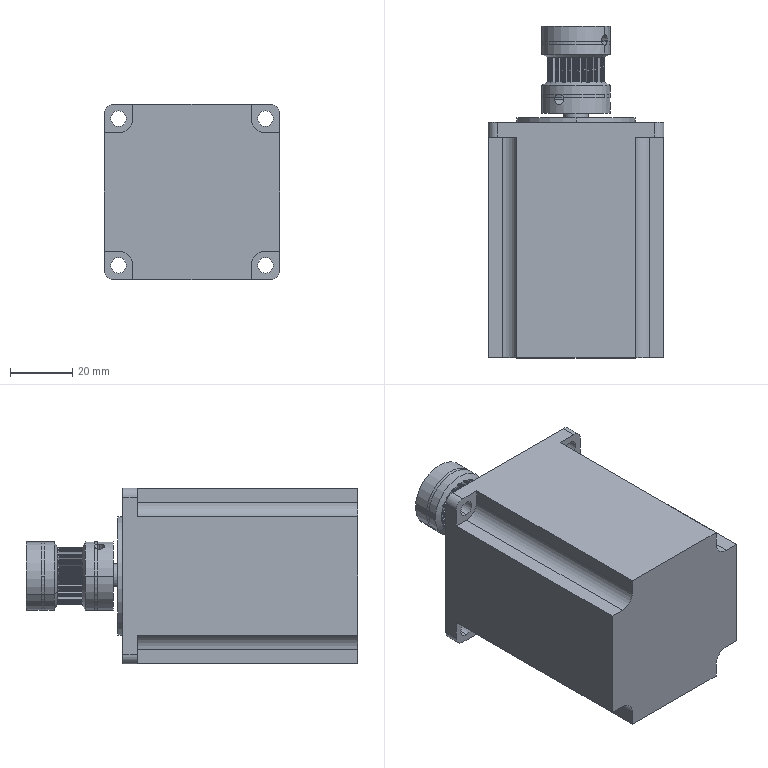Part | SolidWorks | 3 solids | 536 faces | box 56.4 x 106.5 x 56.4 mm | volume 231072 mm3 | cylinder 405 | plane 107 | cone 24 | commonest cylinder face diameters 0.56 x108 0.3 x88 3.95 x84 16.12 x42 18.34 x40 3.3 x8